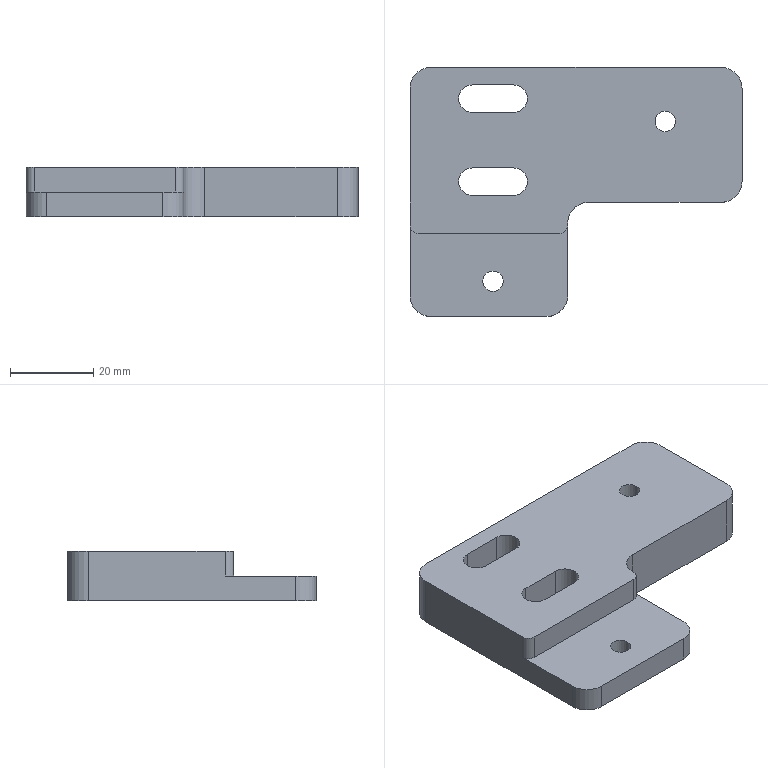NC program | NX | posted with a generic post | part box 80 x 60 x 12 mm
Lines 1 to 18 of 5338:
N10 G17 G21 G94 G90
(FLOOR_WALL , TOOL : D80)
N12 T19 M6
N14 G54
N16 G17 G0 G90 X-88. Y0. S6500 M3
N18 G43 Z30. H19
N20 Z3.
N22 G94 G1 Z0. F1500.
N24 X-85.
N26 X85.
N28 X88.
N30 Z3.
N32 G0 Z30.
N34 M5